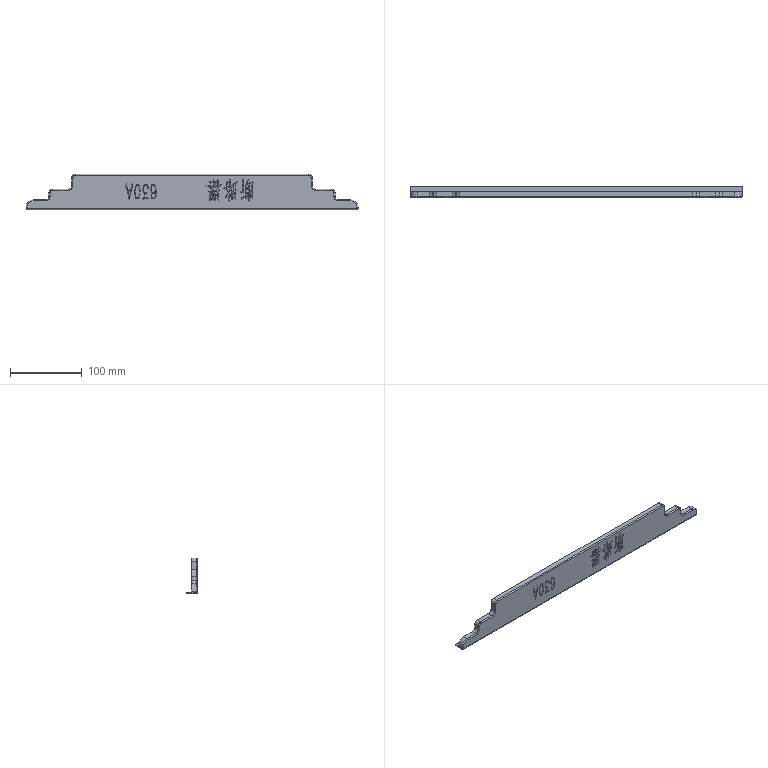Part | STEP file | 1 solid | 585 faces | box 463 x 15 x 50 mm | volume 57863 mm3 | plane 380 | spline 149 | cylinder 44 | torus 10 | sphere 2 | commonest cylinder face diameters 3 x14 10 x8 11 x8 5 x4 9 x4 19 x4